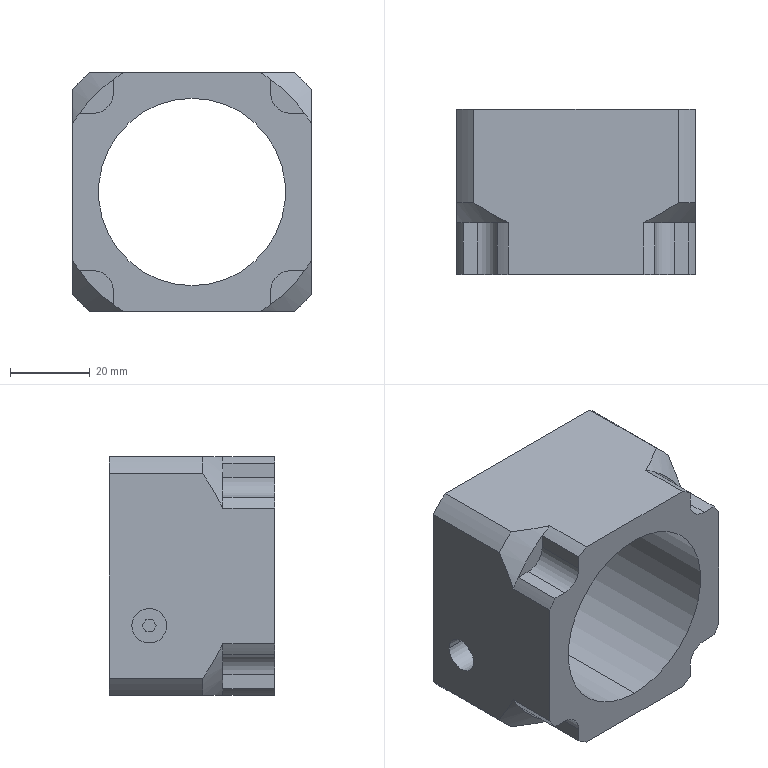Part | NX | 1 solid | 79 faces | box 60 x 41.5 x 60 mm | volume 68848 mm3 | cylinder 32 | plane 31 | cone 14 | torus 2 | commonest cylinder face diameters 3.3 x8 69 x8 10 x4 79 x4 4 x2 8.7 x2